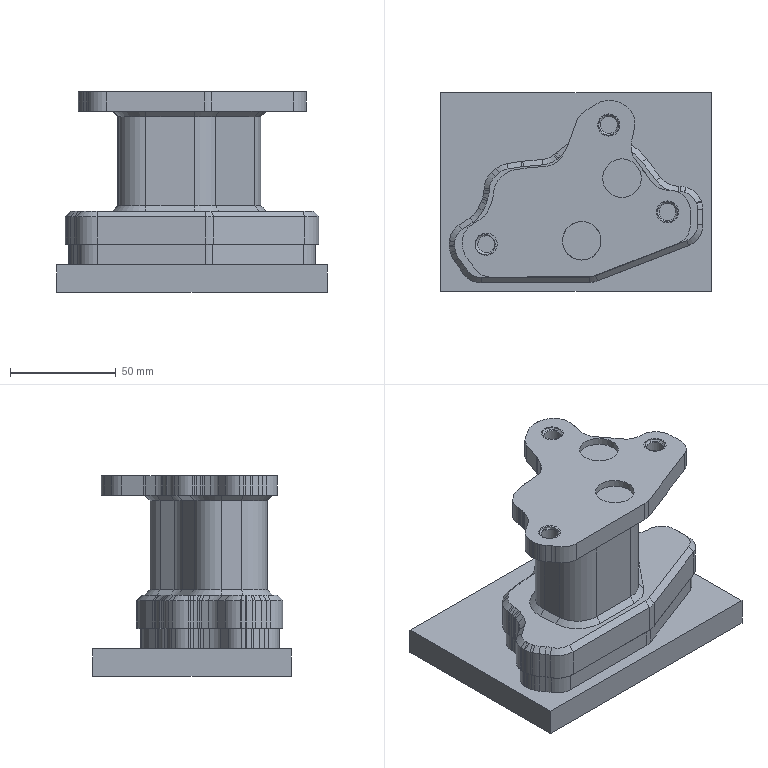CAM job | NX | 3-axis milling, 5-axis milling | part box 128.162 x 94.109 x 95 mm | stock box 128.162 x 94.109 x 95 mm
Tools:
number,name,description,diameter,corner_radius,flute_length,length,flutes
17,C-D20,Milling Tool-5 Parameters,20.0,0.0,50.0,100.0,21
16,J-D16,Milling Tool-5 Parameters,16.0,0.0,40.0,75.0,21
18,C-D10,Milling Tool-5 Parameters,10.0,0.0,30.0,55.0,21
15,J-D10,Milling Tool-5 Parameters,10.0,0.0,30.0,45.0,21
12,J-D4,Milling Tool-5 Parameters,4.0,0.0,10.0,25.0,21
10,J-D6R0.5,Milling Tool-5 Parameters,6.0,0.5,15.0,35.0,21
6,J-D4R2,Milling Tool-Ball Mill,4.0,2.0,10.0,30.0,2
8,J-D2R1,Milling Tool-Ball Mill,2.0,1.0,6.0,6.0,2
34,YD-M6-100,Thread Mill,4.8,0.0,1.0,30.0,33
Operations:
program,operation,operation_type,tool,method,geometry_group,spindle_rpm,surface_speed,feed_per_tooth,feed_cut,feed_plunge,cut_length_mm,path_length_mm,cut_time_min,machine_time_min
A00,DYNROUGH_COPY,SurfaceContour,C-D20,METHOD,1-A,5500.0,345.575,0.0346,4000.0,100.0,4060.766,4935.241,0.644,0.7315
A1,FINISHFACE,FaceMilling,C-D20,METHOD,WP-1,5500.0,345.575,0.013,1500.0,100.0,980.877,1060.677,0.6539,0.6619
A1,DYNROUGH,SurfaceContour,C-D20,METHOD,WP-1,5500.0,345.575,0.0346,4000.0,100.0,26889.616,28712.757,4.78,4.962
A1,NEWFLOORWALL,VolumeBased25DMillingOperation,C-D20,METHOD,WP-1,5500.0,345.575,0.0087,1000.0,100.0,1577.242,1822.042,1.577,1.602
A2,RESTROUGH,CavityMilling,C-D10,METHOD,WP-1,7000.0,100.0,0.1178,3500.0,100.0,17247.192,40362.217,4.928,7.239
A2,RESTROUGH_COPY,CavityMilling,C-D10,METHOD,WP-1,7000.0,100.0,0.1178,3500.0,100.0,19226.99,48068.376,5.493,8.378
A2,RESTROUGH_COPY_1,CavityMilling,C-D10,METHOD,WP-1,7000.0,100.0,0.1178,3500.0,100.0,9962.013,28353.055,2.846,4.685
A2,RESTROUGH_COPY_2,CavityMilling,C-D10,METHOD,WP-1,7000.0,100.0,0.1178,3500.0,100.0,15700.754,33356.499,4.486,6.252
A2,SMALLHOLEROUGH1,CylinderMilling,C-D10,METHOD,WP-1,7000.0,0.0,0.0,1000.0,100.0,1141.389,1343.331,1.141,1.162
A3,SMALLHOLEROUGH1_1,CylinderMilling,J-D4,METHOD,WP-1,7000.0,0.0,0.0,1000.0,100.0,1118.342,1521.939,1.118,1.159
A3,FINISHSMALLHOLE-1,PlanarMilling,J-D4,METHOD,WP-1,7000.0,188.0,0.0,200.0,250.0,110.94,813.778,0.5449,0.6152
A3,FINISHFACE_1,FaceMilling,J-D10,METHOD,WP-1,7000.0,829.0,0.0048,700.0,100.0,985.026,1065.026,1.407,1.415
A3,FINISHLARGEHOLE-1,PlanarMilling,J-D10,METHOD,WP-1,7000.0,188.0,0.0063,400.0,250.0,129.642,332.435,0.3378,0.358
A3,FINISHLARGEHOLE-1_COPY,PlanarMilling,J-D10,METHOD,WP-1,7000.0,188.0,0.0063,400.0,250.0,700.897,807.539,1.759,1.77
A4,FINISHLARGEHOLE-1_COPY_COPY,PlanarMilling,J-D16,METHOD,WP-1,2000.0,100.531,0.0095,400.0,250.0,781.917,1004.789,1.961,1.984
A5,NEWFLOORWALL_1,VolumeBased25DMillingOperation,J-D6R0.5,METHOD,WP-1,8000.0,87.0,0.2143,1000.0,100.0,451.753,660.792,0.4518,0.4727
A5,NEWFLOORWALL_1_COPY,VolumeBased25DMillingOperation,J-D6R0.5,METHOD,WP-1,8000.0,87.0,0.2143,1000.0,100.0,234.747,473.839,0.2347,0.2587
A5,ZLEVELHYBRID,ZLevelMilling,J-D6R0.5,METHOD,1-A,8000.0,122.0,0.0044,2500.0,250.0,88277.644,88761.156,35.454,35.502
A5,ZLEVELHYBRID_COPY,ZLevelMilling,J-D6R0.5,METHOD,1-A,8000.0,122.0,0.0044,2500.0,250.0,92106.333,92787.265,37.108,37.176
A6,FINISHSTEEP,SurfaceContour,J-D4R2,METHOD,WP-1,9000.0,0.0,0.0,3500.0,100.0,4040.698,4275.58,1.155,1.178
A6,ROTARY_DEBURRING,TpMultiAxisDeburring,J-D4R2,METHOD,WP-1,9000.0,0.0,0.0,270.0,90.0,307.884,403.041,1.141,1.151
A6,3AXISDEBURR,TpMultiAxisDeburring,J-D4R2,METHOD,WP-1,9000.0,0.0,0.0,1000.0,90.0,109.276,159.703,0.1099,0.1099
A6,3AXISDEBURR_COPY,TpMultiAxisDeburring,J-D4R2,METHOD,WP-1,9000.0,0.0,0.0,1000.0,90.0,327.049,334.669,0.3274,0.3274
A6,3AXISDEBURR_COPY_1,TpMultiAxisDeburring,J-D4R2,METHOD,1-A,9000.0,0.0,0.0,1000.0,90.0,51.336,427.601,0.0523,0.0523
A7,VARAXISGUIDE,SurfaceContour,J-D2R1,METHOD,WP-1,9000.0,0.0,0.0,2500.0,250.0,11170.164,11331.861,4.485,4.501
A7,VARAXISGUIDE_COPY,SurfaceContour,J-D2R1,METHOD,WP-1,9000.0,0.0,0.0,2500.0,250.0,10408.287,10571.77,4.184,4.2
A7,VARAXISGUIDE_COPY_COPY,SurfaceContour,J-D2R1,METHOD,WP-1,9000.0,0.0,0.0,2500.0,250.0,1848.571,1987.422,0.7586,0.7725
B0,DYNROUGH_1_COPY,SurfaceContour,C-D10,METHOD,2-A,7000.0,0.0,0.0,4000.0,100.0,2292.488,2488.76,0.3474,0.3671
B1,DYNROUGH_1,SurfaceContour,C-D10,METHOD,WP-2,7000.0,0.0,0.0,4000.0,100.0,15147.88,15196.808,3.787,3.792
B1,NEWFLOORWALL_2,VolumeBased25DMillingOperation,J-D10,METHOD,WP-2,8000.0,87.0,0.2143,1000.0,100.0,1711.212,1836.34,1.711,1.724
B-GZ,SMALLHOLEROUGH1_1_COPY,CylinderMilling,J-D4,METHOD,2-A,7000.0,87.965,0.0041,600.0,100.0,1956.272,2373.184,3.26,3.302
B-GZ,M6-THREADMILL,CylinderMilling,YD-M6-100,METHOD,2-A,6000.0,118.0,0.0146,400.0,100.0,351.877,812.222,0.8797,0.9257